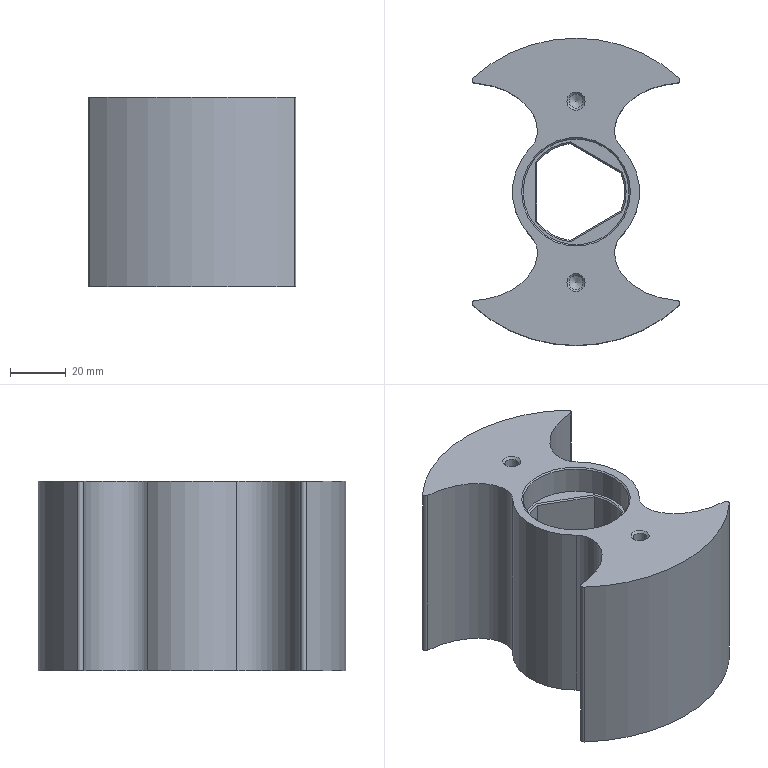NC program | NX | posted with a generic post | part box 74.46 x 110.159 x 68 mm
Lines 14183 to 14265 of 14265:
(PLANAR_MILL_COPY_COPY , TOOL : D6A45)
N28352 T07 M6
N28354 G54
N28356 G17 G0 G90 X-20.135 Y-0.214 S7500 M3
N28358 G43 Z30. H7
N28360 Z1.5
N28362 G94 G1 Z-1.5 F1250.
N28364 G3 X-20.5 Y0. R0.5
N28366 X-20.25 Y-0.25 R0.25
N28368 X-20.5 Y0. R-0.25
N28370 X-20.301 Y-0.084 R0.5
N28372 G1 Z1.5
N28374 G0 Z30.
N28376 X-36.077 Y-28.424
N28378 Z1.5
N28380 G1 Z-1.5
N28382 G3 X-36.644 Y-29.051 R1.
N28384 X-37.342 Y-31.769 R29.394
N28386 X-37.975 Y-36.263 R35.761
N28388 G2 X-41.673 Y-37.527 R2.125
N28390 X-41.673 Y37.527 R56.079
N28392 X-37.975 Y36.263 R2.125
N28394 G3 X-36.693 Y29.203 R34.847
N28396 X-33.8 Y22.749 R25.57
N28398 X-30.744 Y18.91 R21.936
N28400 X-26.874 Y16.095 R15.243
N28402 X-24.268 Y15.111 R12.68
N28404 X-21.582 Y14.826 R9.316
N28406 X-18.973 Y15.385 R7.837
N28408 X-16.807 Y16.81 R6.529
N28410 G2 X16.807 Y16.81 R23.771
N28412 G3 X18.97 Y15.386 R6.529
N28414 X21.575 Y14.826 R7.833
N28416 X24.26 Y15.109 R9.311
N28418 X26.866 Y16.091 R12.665
N28420 X30.622 Y18.792 R15.194
N28422 X33.618 Y22.463 R21.584
N28424 X36.644 Y29.038 R25.349
N28426 X37.975 Y36.263 R34.786
N28428 G2 X41.673 Y37.527 R2.125
N28430 X41.673 Y-37.527 R56.079
N28432 X37.975 Y-36.263 R2.125
N28434 G3 X36.693 Y-29.203 R34.847
N28436 X33.8 Y-22.749 R25.57
N28438 X30.744 Y-18.91 R21.936
N28440 X26.874 Y-16.095 R15.243
N28442 X24.268 Y-15.111 R12.68
N28444 X21.582 Y-14.826 R9.316
N28446 X18.973 Y-15.385 R7.837
N28448 X16.807 Y-16.81 R6.529
N28450 G2 X-16.807 Y-16.81 R23.771
N28452 G3 X-19.55 Y-15.181 R6.554
N28454 X-22.865 Y-14.867 R8.552
N28456 X-26.61 Y-15.956 R10.818
N28458 X-29.972 Y-18.208 R16.126
N28460 X-33.582 Y-22.395 R19.331
N28462 X-36.095 Y-27.436 R26.739
N28464 X-36.644 Y-29.051 R29.394
N28466 X-36.529 Y-29.888 R1.
N28468 G1 Z1.5
N28470 G0 Z30.
N28472 X-0.766 Y-16.943
N28474 Z1.5
N28476 G1 Z-1.5
N28478 G3 X0. Y-17.3 R1.
N28480 X17.3 Y0. R17.3
N28482 X0. Y-17.3 R-17.3
N28484 X0.766 Y-16.943 R1.
N28486 G1 Z1.5
N28488 G0 Z30.
N28490 X20.301 Y-0.084
N28492 Z1.5
N28494 G1 Z-1.5
N28496 G3 X20.5 Y0. R0.5
N28498 X20.25 Y0.25 R0.25
N28500 X20.5 Y0. R-0.25
N28502 X20.135 Y-0.214 R0.5
N28504 G1 Z1.5
N28506 G0 Z30.
N28508 M5
N28510 M2